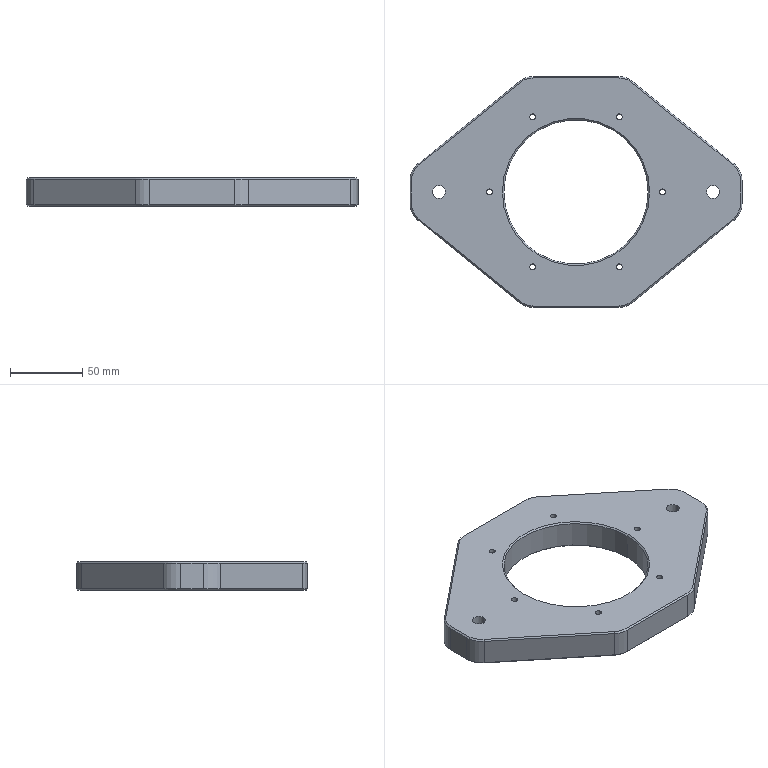Part | SolidWorks | features Chamfer 3, HoleWzd 2, ICE 2, Cut 1, Extrusion 1, Fillet 1 | 1 solid | 82 faces | box 230 x 160 x 20 mm | volume 361707 mm3 | cylinder 30 | plane 28 | cone 24 | commonest cylinder face diameters 4.2 x12 30 x8 9 x4 20.5 x4 100 x2